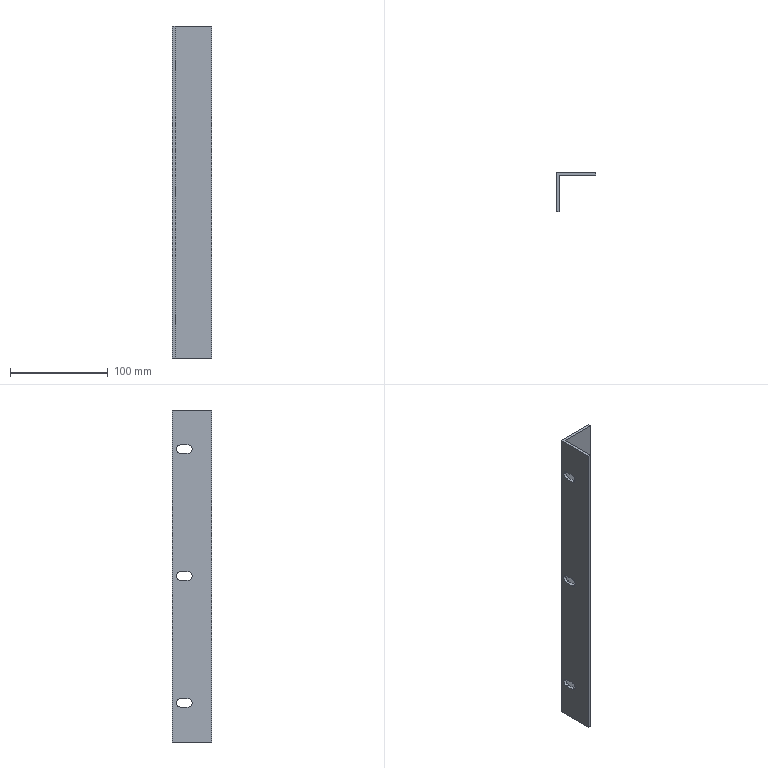Part | STEP file | PN_0062 (belt pad block) | 1 solid | 23 faces | box 40 x 40 x 340 mm | volume 77417 mm3 | plane 14 | cylinder 9 | commonest cylinder face diameters 8.5 x9